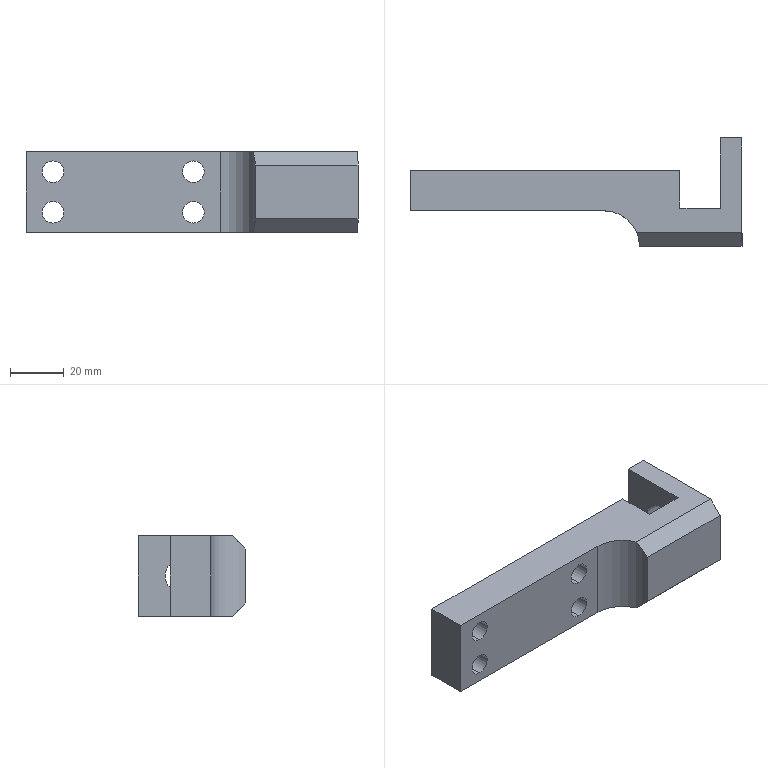Part | SolidWorks | features BaseBody 1 | 1 solid | 24 faces | box 123 x 40 x 30 mm | volume 62963 mm3 | plane 13 | cylinder 11 | commonest cylinder face diameters 8 x8 12 x2 26 x1
STEP:
#1=CARTESIAN_POINT('',(-340.,-80.,148.121));
#2=VERTEX_POINT('',#1);
#3=CARTESIAN_POINT('',(-340.,-80.,156.121));
#4=VERTEX_POINT('',#3);
#5=CARTESIAN_POINT('',(-340.,-80.,152.121));
#6=DIRECTION('',(0.,1.,0.));
#7=DIRECTION('',(0.,0.,-1.));
#8=AXIS2_PLACEMENT_3D('',#5,#6,#7);
#9=CIRCLE('',#8,4.);
#10=EDGE_CURVE('',#2,#4,#9,.T.);
#11=ORIENTED_EDGE('',*,*,#10,.T.);
#12=CARTESIAN_POINT('',(-340.,-95.,156.121));
#13=VERTEX_POINT('',#12);
#14=CARTESIAN_POINT('',(-340.,-95.,156.121));
#15=DIRECTION('',(0.,-1.,0.));
#16=VECTOR('',#15,1000.);
#17=LINE('',#14,#16);
#18=EDGE_CURVE('',#4,#13,#17,.T.);
#19=ORIENTED_EDGE('',*,*,#18,.T.);
#20=CARTESIAN_POINT('',(-340.,-95.,148.121));
#21=VERTEX_POINT('',#20);
#22=CARTESIAN_POINT('',(-340.,-95.,152.121));
#23=DIRECTION('',(0.,1.,0.));
#24=DIRECTION('',(0.,0.,-1.));
#25=AXIS2_PLACEMENT_3D('',#22,#23,#24);
#26=CIRCLE('',#25,4.);
#27=EDGE_CURVE('',#21,#13,#26,.T.);
#28=ORIENTED_EDGE('',*,*,#27,.F.);
#29=CARTESIAN_POINT('',(-340.,-95.,148.121));
#30=DIRECTION('',(0.,-1.,0.));
#31=VECTOR('',#30,1000.);
#32=LINE('',#29,#31);
#33=EDGE_CURVE('',#2,#21,#32,.T.);
#34=ORIENTED_EDGE('',*,*,#33,.F.);
#35=EDGE_LOOP('',(#11,#19,#28,#34));
#36=FACE_OUTER_BOUND('',#35,.T.);
#37=CARTESIAN_POINT('',(-340.,-95.,152.121));
#38=DIRECTION('',(0.,-1.,0.));
#39=DIRECTION('',(0.,0.,-1.));
#40=AXIS2_PLACEMENT_3D('',#37,#38,#39);
#41=CYLINDRICAL_SURFACE('',#40,4.);
#42=ADVANCED_FACE('',(#36),#41,.F.);
#43=CARTESIAN_POINT('',(-340.,-80.,133.121));
#44=VERTEX_POINT('',#43);
#45=CARTESIAN_POINT('',(-340.,-80.,141.121));
#46=VERTEX_POINT('',#45);
#47=CARTESIAN_POINT('',(-340.,-80.,137.121));
#48=DIRECTION('',(0.,1.,0.));
#49=DIRECTION('',(0.,0.,-1.));
#50=AXIS2_PLACEMENT_3D('',#47,#48,#49);
#51=CIRCLE('',#50,4.);
#52=EDGE_CURVE('',#44,#46,#51,.T.);
#53=ORIENTED_EDGE('',*,*,#52,.T.);
#54=CARTESIAN_POINT('',(-340.,-95.,141.121));
#55=VERTEX_POINT('',#54);
#56=CARTESIAN_POINT('',(-340.,-95.,141.121));
#57=DIRECTION('',(0.,-1.,0.));
#58=VECTOR('',#57,1000.);
#59=LINE('',#56,#58);
#60=EDGE_CURVE('',#46,#55,#59,.T.);
#61=ORIENTED_EDGE('',*,*,#60,.T.);
#62=CARTESIAN_POINT('',(-340.,-95.,133.121));
#63=VERTEX_POINT('',#62);
#64=CARTESIAN_POINT('',(-340.,-95.,137.121));
#65=DIRECTION('',(0.,1.,0.));
#66=DIRECTION('',(0.,0.,-1.));
#67=AXIS2_PLACEMENT_3D('',#64,#65,#66);
#68=CIRCLE('',#67,4.);
#69=EDGE_CURVE('',#63,#55,#68,.T.);
#70=ORIENTED_EDGE('',*,*,#69,.F.);
#71=CARTESIAN_POINT('',(-340.,-95.,133.121));
#72=DIRECTION('',(0.,-1.,0.));
#73=VECTOR('',#72,1000.);
#74=LINE('',#71,#73);
#75=EDGE_CURVE('',#44,#63,#74,.T.);
#76=ORIENTED_EDGE('',*,*,#75,.F.);
#77=EDGE_LOOP('',(#53,#61,#70,#76));
#78=FACE_OUTER_BOUND('',#77,.T.);
#79=CARTESIAN_POINT('',(-340.,-95.,137.121));
#80=DIRECTION('',(0.,-1.,0.));
#81=DIRECTION('',(0.,0.,-1.));
#82=AXIS2_PLACEMENT_3D('',#79,#80,#81);
#83=CYLINDRICAL_SURFACE('',#82,4.);
#84=ADVANCED_FACE('',(#78),#83,.F.);
#85=CARTESIAN_POINT('',(-288.,-80.,133.121));
#86=VERTEX_POINT('',#85);
#87=CARTESIAN_POINT('',(-288.,-80.,141.121));
#88=VERTEX_POINT('',#87);
#89=CARTESIAN_POINT('',(-288.,-80.,137.121));
#90=DIRECTION('',(0.,1.,0.));
#91=DIRECTION('',(0.,0.,-1.));
#92=AXIS2_PLACEMENT_3D('',#89,#90,#91);
#93=CIRCLE('',#92,4.);
#94=EDGE_CURVE('',#86,#88,#93,.T.);
#95=ORIENTED_EDGE('',*,*,#94,.T.);
#96=CARTESIAN_POINT('',(-288.,-95.,141.121));
#97=VERTEX_POINT('',#96);
#98=CARTESIAN_POINT('',(-288.,-95.,141.121));
#99=DIRECTION('',(0.,-1.,0.));
#100=VECTOR('',#99,1000.);
#101=LINE('',#98,#100);
#102=EDGE_CURVE('',#88,#97,#101,.T.);
#103=ORIENTED_EDGE('',*,*,#102,.T.);
#104=CARTESIAN_POINT('',(-288.,-95.,133.121));
#105=VERTEX_POINT('',#104);
#106=CARTESIAN_POINT('',(-288.,-95.,137.121));
#107=DIRECTION('',(0.,1.,0.));
#108=DIRECTION('',(0.,0.,-1.));
#109=AXIS2_PLACEMENT_3D('',#106,#107,#108);
#110=CIRCLE('',#109,4.);
#111=EDGE_CURVE('',#105,#97,#110,.T.);
#112=ORIENTED_EDGE('',*,*,#111,.F.);
#113=CARTESIAN_POINT('',(-288.,-95.,133.121));
#114=DIRECTION('',(0.,-1.,0.));
#115=VECTOR('',#114,1000.);
#116=LINE('',#113,#115);
#117=EDGE_CURVE('',#86,#105,#116,.T.);
#118=ORIENTED_EDGE('',*,*,#117,.F.);
#119=EDGE_LOOP('',(#95,#103,#112,#118));
#120=FACE_OUTER_BOUND('',#119,.T.);
#121=CARTESIAN_POINT('',(-288.,-95.,137.121));
#122=DIRECTION('',(0.,-1.,0.));
#123=DIRECTION('',(0.,0.,-1.));
#124=AXIS2_PLACEMENT_3D('',#121,#122,#123);
#125=CYLINDRICAL_SURFACE('',#124,4.);
#126=ADVANCED_FACE('',(#120),#125,.F.);
#127=CARTESIAN_POINT('',(-288.,-80.,148.121));
#128=VERTEX_POINT('',#127);
#129=CARTESIAN_POINT('',(-288.,-80.,156.121));
#130=VERTEX_POINT('',#129);
#131=CARTESIAN_POINT('',(-288.,-80.,152.121));
#132=DIRECTION('',(0.,1.,0.));
#133=DIRECTION('',(0.,0.,-1.));
#134=AXIS2_PLACEMENT_3D('',#131,#132,#133);
#135=CIRCLE('',#134,4.);
#136=EDGE_CURVE('',#128,#130,#135,.T.);
#137=ORIENTED_EDGE('',*,*,#136,.T.);
#138=CARTESIAN_POINT('',(-288.,-95.,156.121));
#139=VERTEX_POINT('',#138);
#140=CARTESIAN_POINT('',(-288.,-95.,156.121));
#141=DIRECTION('',(0.,-1.,0.));
#142=VECTOR('',#141,1000.);
#143=LINE('',#140,#142);
#144=EDGE_CURVE('',#130,#139,#143,.T.);
#145=ORIENTED_EDGE('',*,*,#144,.T.);
#146=CARTESIAN_POINT('',(-288.,-95.,148.121));
#147=VERTEX_POINT('',#146);
#148=CARTESIAN_POINT('',(-288.,-95.,152.121));
#149=DIRECTION('',(0.,1.,0.));
#150=DIRECTION('',(0.,0.,-1.));
#151=AXIS2_PLACEMENT_3D('',#148,#149,#150);
#152=CIRCLE('',#151,4.);
#153=EDGE_CURVE('',#147,#139,#152,.T.);
#154=ORIENTED_EDGE('',*,*,#153,.F.);
#155=CARTESIAN_POINT('',(-288.,-95.,148.121));
#156=DIRECTION('',(0.,-1.,0.));
#157=VECTOR('',#156,1000.);
#158=LINE('',#155,#157);
#159=EDGE_CURVE('',#128,#147,#158,.T.);
#160=ORIENTED_EDGE('',*,*,#159,.F.);
#161=EDGE_LOOP('',(#137,#145,#154,#160));
#162=FACE_OUTER_BOUND('',#161,.T.);
#163=CARTESIAN_POINT('',(-288.,-95.,152.121));
#164=DIRECTION('',(0.,-1.,0.));
#165=DIRECTION('',(0.,0.,-1.));
#166=AXIS2_PLACEMENT_3D('',#163,#164,#165);
#167=CYLINDRICAL_SURFACE('',#166,4.);
#168=ADVANCED_FACE('',(#162),#167,.F.);
#169=CARTESIAN_POINT('',(-235.,-84.,138.621));
#170=VERTEX_POINT('',#169);
#171=CARTESIAN_POINT('',(-235.,-84.,150.621));
#172=VERTEX_POINT('',#171);
#173=CARTESIAN_POINT('',(-235.,-84.,144.621));
#174=DIRECTION('',(-1.,0.,0.));
#175=DIRECTION('',(0.,0.,-1.));
#176=AXIS2_PLACEMENT_3D('',#173,#174,#175);
#177=CIRCLE('',#176,6.);
#178=EDGE_CURVE('',#170,#172,#177,.T.);
#179=ORIENTED_EDGE('',*,*,#178,.T.);
#180=CARTESIAN_POINT('',(-227.,-84.,150.621));
#181=VERTEX_POINT('',#180);
#182=CARTESIAN_POINT('',(-251.971,-84.,150.621));
#183=DIRECTION('',(1.,0.,0.));
#184=VECTOR('',#183,1000.);
#185=LINE('',#182,#184);
#186=EDGE_CURVE('',#172,#181,#185,.T.);
#187=ORIENTED_EDGE('',*,*,#186,.T.);
#188=CARTESIAN_POINT('',(-227.,-84.,138.621));
#189=VERTEX_POINT('',#188);
#190=CARTESIAN_POINT('',(-227.,-84.,144.621));
#191=DIRECTION('',(1.,0.,0.));
#192=DIRECTION('',(0.,0.,-1.));
#193=AXIS2_PLACEMENT_3D('',#190,#191,#192);
#194=CIRCLE('',#193,6.);
#195=EDGE_CURVE('',#181,#189,#194,.T.);
#196=ORIENTED_EDGE('',*,*,#195,.T.);
#197=CARTESIAN_POINT('',(-251.971,-84.,138.621));
#198=DIRECTION('',(1.,0.,0.));
#199=VECTOR('',#198,1000.);
#200=LINE('',#197,#199);
#201=EDGE_CURVE('',#170,#189,#200,.T.);
#202=ORIENTED_EDGE('',*,*,#201,.F.);
#203=EDGE_LOOP('',(#179,#187,#196,#202));
#204=FACE_OUTER_BOUND('',#203,.T.);
#205=CARTESIAN_POINT('',(-251.971,-84.,144.621));
#206=DIRECTION('',(1.,0.,0.));
#207=DIRECTION('',(0.,0.,-1.));
#208=AXIS2_PLACEMENT_3D('',#205,#206,#207);
#209=CYLINDRICAL_SURFACE('',#208,6.);
#210=ADVANCED_FACE('',(#204),#209,.F.);
#211=CARTESIAN_POINT('',(-350.,-80.,159.621));
#212=VERTEX_POINT('',#211);
#213=CARTESIAN_POINT('',(-350.,-80.,129.621));
#214=VERTEX_POINT('',#213);
#215=CARTESIAN_POINT('',(-350.,-80.,159.621));
#216=DIRECTION('',(0.,0.,-1.));
#217=VECTOR('',#216,1000.);
#218=LINE('',#215,#217);
#219=EDGE_CURVE('',#212,#214,#218,.T.);
#220=ORIENTED_EDGE('',*,*,#219,.F.);
#221=CARTESIAN_POINT('',(-250.,-80.,159.621));
#222=VERTEX_POINT('',#221);
#223=CARTESIAN_POINT('',(-350.,-80.,159.621));
#224=DIRECTION('',(-1.,0.,0.));
#225=VECTOR('',#224,1000.);
#226=LINE('',#223,#225);
#227=EDGE_CURVE('',#222,#212,#226,.T.);
#228=ORIENTED_EDGE('',*,*,#227,.F.);
#229=CARTESIAN_POINT('',(-250.,-80.,129.621));
#230=VERTEX_POINT('',#229);
#231=CARTESIAN_POINT('',(-250.,-80.,159.621));
#232=DIRECTION('',(0.,0.,1.));
#233=VECTOR('',#232,1000.);
#234=LINE('',#231,#233);
#235=EDGE_CURVE('',#230,#222,#234,.T.);
#236=ORIENTED_EDGE('',*,*,#235,.F.);
#237=CARTESIAN_POINT('',(-350.,-80.,129.621));
#238=DIRECTION('',(1.,0.,0.));
#239=VECTOR('',#238,1000.);
#240=LINE('',#237,#239);
#241=EDGE_CURVE('',#214,#230,#240,.T.);
#242=ORIENTED_EDGE('',*,*,#241,.F.);
#243=EDGE_LOOP('',(#220,#228,#236,#242));
#244=FACE_OUTER_BOUND('',#243,.T.);
#245=ORIENTED_EDGE('',*,*,#10,.F.);
#246=CARTESIAN_POINT('',(-340.,-80.,152.121));
#247=DIRECTION('',(0.,1.,0.));
#248=DIRECTION('',(0.,0.,-1.));
#249=AXIS2_PLACEMENT_3D('',#246,#247,#248);
#250=CIRCLE('',#249,4.);
#251=EDGE_CURVE('',#4,#2,#250,.T.);
#252=ORIENTED_EDGE('',*,*,#251,.F.);
#253=EDGE_LOOP('',(#245,#252));
#254=FACE_BOUND('',#253,.T.);
#255=ORIENTED_EDGE('',*,*,#52,.F.);
#256=CARTESIAN_POINT('',(-340.,-80.,137.121));
#257=DIRECTION('',(0.,1.,0.));
#258=DIRECTION('',(0.,0.,-1.));
#259=AXIS2_PLACEMENT_3D('',#256,#257,#258);
#260=CIRCLE('',#259,4.);
#261=EDGE_CURVE('',#46,#44,#260,.T.);
#262=ORIENTED_EDGE('',*,*,#261,.F.);
#263=EDGE_LOOP('',(#255,#262));
#264=FACE_BOUND('',#263,.T.);
#265=ORIENTED_EDGE('',*,*,#94,.F.);
#266=CARTESIAN_POINT('',(-288.,-80.,137.121));
#267=DIRECTION('',(0.,1.,0.));
#268=DIRECTION('',(0.,0.,-1.));
#269=AXIS2_PLACEMENT_3D('',#266,#267,#268);
#270=CIRCLE('',#269,4.);
#271=EDGE_CURVE('',#88,#86,#270,.T.);
#272=ORIENTED_EDGE('',*,*,#271,.F.);
#273=EDGE_LOOP('',(#265,#272));
#274=FACE_BOUND('',#273,.T.);
#275=ORIENTED_EDGE('',*,*,#136,.F.);
#276=CARTESIAN_POINT('',(-288.,-80.,152.121));
#277=DIRECTION('',(0.,1.,0.));
#278=DIRECTION('',(0.,0.,-1.));
#279=AXIS2_PLACEMENT_3D('',#276,#277,#278);
#280=CIRCLE('',#279,4.);
#281=EDGE_CURVE('',#130,#128,#280,.T.);
#282=ORIENTED_EDGE('',*,*,#281,.F.);
#283=EDGE_LOOP('',(#275,#282));
#284=FACE_BOUND('',#283,.T.);
#285=CARTESIAN_POINT('',(-350.,-80.,159.621));
#286=DIRECTION('',(0.,-1.,0.));
#287=DIRECTION('',(0.,0.,-1.));
#288=AXIS2_PLACEMENT_3D('',#285,#286,#287);
#289=PLANE('',#288);
#290=ADVANCED_FACE('',(#244,#254,#264,#274,#284),#289,.F.);
#291=CARTESIAN_POINT('',(-266.,-103.,129.621));
#292=VERTEX_POINT('',#291);
#293=CARTESIAN_POINT('',(-227.,-103.,129.621));
#294=VERTEX_POINT('',#293);
#295=CARTESIAN_POINT('',(-251.867,-103.,129.621));
#296=DIRECTION('',(1.,0.,0.));
#297=VECTOR('',#296,1000.);
#298=LINE('',#295,#297);
#299=EDGE_CURVE('',#292,#294,#298,.T.);
#300=ORIENTED_EDGE('',*,*,#299,.F.);
#301=CARTESIAN_POINT('',(-278.,-95.,129.621));
#302=VERTEX_POINT('',#301);
#303=CARTESIAN_POINT('',(-278.,-108.,129.621));
#304=DIRECTION('',(0.,0.,-1.));
#305=DIRECTION('',(1.,0.,0.));
#306=AXIS2_PLACEMENT_3D('',#303,#304,#305);
#307=CIRCLE('',#306,13.);
#308=EDGE_CURVE('',#302,#292,#307,.T.);
#309=ORIENTED_EDGE('',*,*,#308,.F.);
#310=CARTESIAN_POINT('',(-350.,-95.,129.621));
#311=VERTEX_POINT('',#310);
#312=CARTESIAN_POINT('',(-251.867,-95.,129.621));
#313=DIRECTION('',(1.,0.,0.));
#314=VECTOR('',#313,1000.);
#315=LINE('',#312,#314);
#316=EDGE_CURVE('',#311,#302,#315,.T.);
#317=ORIENTED_EDGE('',*,*,#316,.F.);
#318=CARTESIAN_POINT('',(-350.,-82.6,129.621));
#319=DIRECTION('',(0.,-1.,0.));
#320=VECTOR('',#319,1000.);
#321=LINE('',#318,#320);
#322=EDGE_CURVE('',#214,#311,#321,.T.);
#323=ORIENTED_EDGE('',*,*,#322,.F.);
#324=ORIENTED_EDGE('',*,*,#241,.T.);
#325=CARTESIAN_POINT('',(-250.,-94.,129.621));
#326=VERTEX_POINT('',#325);
#327=CARTESIAN_POINT('',(-250.,-82.6,129.621));
#328=DIRECTION('',(0.,1.,0.));
#329=VECTOR('',#328,1000.);
#330=LINE('',#327,#329);
#331=EDGE_CURVE('',#326,#230,#330,.T.);
#332=ORIENTED_EDGE('',*,*,#331,.F.);
#333=CARTESIAN_POINT('',(-235.,-94.,129.621));
#334=VERTEX_POINT('',#333);
#335=CARTESIAN_POINT('',(-251.867,-94.,129.621));
#336=DIRECTION('',(-1.,0.,0.));
#337=VECTOR('',#336,1000.);
#338=LINE('',#335,#337);
#339=EDGE_CURVE('',#334,#326,#338,.T.);
#340=ORIENTED_EDGE('',*,*,#339,.F.);
#341=CARTESIAN_POINT('',(-235.,-68.,129.621));
#342=VERTEX_POINT('',#341);
#343=CARTESIAN_POINT('',(-235.,-82.6,129.621));
#344=DIRECTION('',(0.,-1.,0.));
#345=VECTOR('',#344,1000.);
#346=LINE('',#343,#345);
#347=EDGE_CURVE('',#342,#334,#346,.T.);
#348=ORIENTED_EDGE('',*,*,#347,.F.);
#349=CARTESIAN_POINT('',(-227.,-68.,129.621));
#350=VERTEX_POINT('',#349);
#351=CARTESIAN_POINT('',(-251.867,-68.,129.621));
#352=DIRECTION('',(-1.,0.,0.));
#353=VECTOR('',#352,1000.);
#354=LINE('',#351,#353);
#355=EDGE_CURVE('',#350,#342,#354,.T.);
#356=ORIENTED_EDGE('',*,*,#355,.F.);
#357=CARTESIAN_POINT('',(-227.,-82.6,129.621));
#358=DIRECTION('',(0.,1.,0.));
#359=VECTOR('',#358,1000.);
#360=LINE('',#357,#359);
#361=EDGE_CURVE('',#294,#350,#360,.T.);
#362=ORIENTED_EDGE('',*,*,#361,.F.);
#363=EDGE_LOOP('',(#300,#309,#317,#323,#324,#332,#340,#348,#356,#362));
#364=FACE_OUTER_BOUND('',#363,.T.);
#365=CARTESIAN_POINT('',(-251.867,-82.6,129.621));
#366=DIRECTION('',(0.,0.,1.));
#367=DIRECTION('',(1.,0.,0.));
#368=AXIS2_PLACEMENT_3D('',#365,#366,#367);
#369=PLANE('',#368);
#370=ADVANCED_FACE('',(#364),#369,.F.);
#371=CARTESIAN_POINT('',(-350.,-95.,159.621));
#372=VERTEX_POINT('',#371);
#373=CARTESIAN_POINT('',(-350.,-95.,159.621));
#374=DIRECTION('',(0.,0.,-1.));
#375=VECTOR('',#374,1000.);
#376=LINE('',#373,#375);
#377=EDGE_CURVE('',#372,#311,#376,.T.);
#378=ORIENTED_EDGE('',*,*,#377,.F.);
#379=CARTESIAN_POINT('',(-350.,-80.,159.621));
#380=DIRECTION('',(0.,-1.,0.));
#381=VECTOR('',#380,1000.);
#382=LINE('',#379,#381);
#383=EDGE_CURVE('',#212,#372,#382,.T.);
#384=ORIENTED_EDGE('',*,*,#383,.F.);
#385=ORIENTED_EDGE('',*,*,#219,.T.);
#386=ORIENTED_EDGE('',*,*,#322,.T.);
#387=EDGE_LOOP('',(#378,#384,#385,#386));
#388=FACE_OUTER_BOUND('',#387,.T.);
#389=CARTESIAN_POINT('',(-350.,-80.,159.621));
#390=DIRECTION('',(1.,0.,0.));
#391=DIRECTION('',(0.,0.,-1.));
#392=AXIS2_PLACEMENT_3D('',#389,#390,#391);
#393=PLANE('',#392);
#394=ADVANCED_FACE('',(#388),#393,.F.);
#395=ORIENTED_EDGE('',*,*,#383,.T.);
#396=CARTESIAN_POINT('',(-278.,-95.,159.621));
#397=VERTEX_POINT('',#396);
#398=CARTESIAN_POINT('',(-251.867,-95.,159.621));
#399=DIRECTION('',(1.,0.,0.));
#400=VECTOR('',#399,1000.);
#401=LINE('',#398,#400);
#402=EDGE_CURVE('',#372,#397,#401,.T.);
#403=ORIENTED_EDGE('',*,*,#402,.T.);
#404=CARTESIAN_POINT('',(-266.,-103.,159.621));
#405=VERTEX_POINT('',#404);
#406=CARTESIAN_POINT('',(-278.,-108.,159.621));
#407=DIRECTION('',(0.,0.,-1.));
#408=DIRECTION('',(1.,0.,0.));
#409=AXIS2_PLACEMENT_3D('',#406,#407,#408);
#410=CIRCLE('',#409,13.);
#411=EDGE_CURVE('',#397,#405,#410,.T.);
#412=ORIENTED_EDGE('',*,*,#411,.T.);
#413=CARTESIAN_POINT('',(-227.,-103.,159.621));
#414=VERTEX_POINT('',#413);
#415=CARTESIAN_POINT('',(-251.867,-103.,159.621));
#416=DIRECTION('',(1.,0.,0.));
#417=VECTOR('',#416,1000.);
#418=LINE('',#415,#417);
#419=EDGE_CURVE('',#405,#414,#418,.T.);
#420=ORIENTED_EDGE('',*,*,#419,.T.);
#421=CARTESIAN_POINT('',(-227.,-68.,159.621));
#422=VERTEX_POINT('',#421);
#423=CARTESIAN_POINT('',(-227.,-82.6,159.621));
#424=DIRECTION('',(0.,1.,0.));
#425=VECTOR('',#424,1000.);
#426=LINE('',#423,#425);
#427=EDGE_CURVE('',#414,#422,#426,.T.);
#428=ORIENTED_EDGE('',*,*,#427,.T.);
#429=CARTESIAN_POINT('',(-235.,-68.,159.621));
#430=VERTEX_POINT('',#429);
#431=CARTESIAN_POINT('',(-251.867,-68.,159.621));
#432=DIRECTION('',(-1.,0.,0.));
#433=VECTOR('',#432,1000.);
#434=LINE('',#431,#433);
#435=EDGE_CURVE('',#422,#430,#434,.T.);
#436=ORIENTED_EDGE('',*,*,#435,.T.);
#437=CARTESIAN_POINT('',(-235.,-94.,159.621));
#438=VERTEX_POINT('',#437);
#439=CARTESIAN_POINT('',(-235.,-82.6,159.621));
#440=DIRECTION('',(0.,-1.,0.));
#441=VECTOR('',#440,1000.);
#442=LINE('',#439,#441);
#443=EDGE_CURVE('',#430,#438,#442,.T.);
#444=ORIENTED_EDGE('',*,*,#443,.T.);
#445=CARTESIAN_POINT('',(-250.,-94.,159.621));
#446=VERTEX_POINT('',#445);
#447=CARTESIAN_POINT('',(-251.867,-94.,159.621));
#448=DIRECTION('',(-1.,0.,0.));
#449=VECTOR('',#448,1000.);
#450=LINE('',#447,#449);
#451=EDGE_CURVE('',#438,#446,#450,.T.);
#452=ORIENTED_EDGE('',*,*,#451,.T.);
#453=CARTESIAN_POINT('',(-250.,-82.6,159.621));
#454=DIRECTION('',(0.,1.,0.));
#455=VECTOR('',#454,1000.);
#456=LINE('',#453,#455);
#457=EDGE_CURVE('',#446,#222,#456,.T.);
#458=ORIENTED_EDGE('',*,*,#457,.T.);
#459=ORIENTED_EDGE('',*,*,#227,.T.);
#460=EDGE_LOOP('',(#395,#403,#412,#420,#428,#436,#444,#452,#458,#459));
#461=FACE_OUTER_BOUND('',#460,.T.);
#462=CARTESIAN_POINT('',(-251.867,-82.6,159.621));
#463=DIRECTION('',(0.,0.,1.));
#464=DIRECTION('',(1.,0.,0.));
#465=AXIS2_PLACEMENT_3D('',#462,#463,#464);
#466=PLANE('',#465);
#467=ADVANCED_FACE('',(#461),#466,.T.);
#468=ORIENTED_EDGE('',*,*,#235,.T.);
#469=ORIENTED_EDGE('',*,*,#457,.F.);
#470=CARTESIAN_POINT('',(-250.,-94.,159.621));
#471=DIRECTION('',(0.,0.,1.));
#472=VECTOR('',#471,1000.);
#473=LINE('',#470,#472);
#474=EDGE_CURVE('',#326,#446,#473,.T.);
#475=ORIENTED_EDGE('',*,*,#474,.F.);
#476=ORIENTED_EDGE('',*,*,#331,.T.);
#477=EDGE_LOOP('',(#468,#469,#475,#476));
#478=FACE_OUTER_BOUND('',#477,.T.);
#479=CARTESIAN_POINT('',(-250.,-80.,159.621));
#480=DIRECTION('',(-1.,0.,0.));
#481=DIRECTION('',(0.,0.,1.));
#482=AXIS2_PLACEMENT_3D('',#479,#480,#481);
#483=PLANE('',#482);
#484=ADVANCED_FACE('',(#478),#483,.F.);
#485=ORIENTED_EDGE('',*,*,#18,.F.);
#486=ORIENTED_EDGE('',*,*,#251,.T.);
#487=ORIENTED_EDGE('',*,*,#33,.T.);
#488=CARTESIAN_POINT('',(-340.,-95.,152.121));
#489=DIRECTION('',(0.,1.,0.));
#490=DIRECTION('',(0.,0.,-1.));
#491=AXIS2_PLACEMENT_3D('',#488,#489,#490);
#492=CIRCLE('',#491,4.);
#493=EDGE_CURVE('',#13,#21,#492,.T.);
#494=ORIENTED_EDGE('',*,*,#493,.F.);
#495=EDGE_LOOP('',(#485,#486,#487,#494));
#496=FACE_OUTER_BOUND('',#495,.T.);
#497=CARTESIAN_POINT('',(-340.,-95.,152.121));
#498=DIRECTION('',(0.,-1.,0.));
#499=DIRECTION('',(0.,0.,-1.));
#500=AXIS2_PLACEMENT_3D('',#497,#498,#499);
#501=CYLINDRICAL_SURFACE('',#500,4.);
#502=ADVANCED_FACE('',(#496),#501,.F.);
#503=ORIENTED_EDGE('',*,*,#60,.F.);
#504=ORIENTED_EDGE('',*,*,#261,.T.);
#505=ORIENTED_EDGE('',*,*,#75,.T.);
#506=CARTESIAN_POINT('',(-340.,-95.,137.121));
#507=DIRECTION('',(0.,1.,0.));
#508=DIRECTION('',(0.,0.,-1.));
#509=AXIS2_PLACEMENT_3D('',#506,#507,#508);
#510=CIRCLE('',#509,4.);
#511=EDGE_CURVE('',#55,#63,#510,.T.);
#512=ORIENTED_EDGE('',*,*,#511,.F.);
#513=EDGE_LOOP('',(#503,#504,#505,#512));
#514=FACE_OUTER_BOUND('',#513,.T.);
#515=CARTESIAN_POINT('',(-340.,-95.,137.121));
#516=DIRECTION('',(0.,-1.,0.));
#517=DIRECTION('',(0.,0.,-1.));
#518=AXIS2_PLACEMENT_3D('',#515,#516,#517);
#519=CYLINDRICAL_SURFACE('',#518,4.);
#520=ADVANCED_FACE('',(#514),#519,.F.);
#521=ORIENTED_EDGE('',*,*,#102,.F.);
#522=ORIENTED_EDGE('',*,*,#271,.T.);
#523=ORIENTED_EDGE('',*,*,#117,.T.);
#524=CARTESIAN_POINT('',(-288.,-95.,137.121));
#525=DIRECTION('',(0.,1.,0.));
#526=DIRECTION('',(0.,0.,-1.));
#527=AXIS2_PLACEMENT_3D('',#524,#525,#526);
#528=CIRCLE('',#527,4.);
#529=EDGE_CURVE('',#97,#105,#528,.T.);
#530=ORIENTED_EDGE('',*,*,#529,.F.);
#531=EDGE_LOOP('',(#521,#522,#523,#530));
#532=FACE_OUTER_BOUND('',#531,.T.);
#533=CARTESIAN_POINT('',(-288.,-95.,137.121));
#534=DIRECTION('',(0.,-1.,0.));
#535=DIRECTION('',(0.,0.,-1.));
#536=AXIS2_PLACEMENT_3D('',#533,#534,#535);
#537=CYLINDRICAL_SURFACE('',#536,4.);
#538=ADVANCED_FACE('',(#532),#537,.F.);
#539=ORIENTED_EDGE('',*,*,#144,.F.);
#540=ORIENTED_EDGE('',*,*,#281,.T.);
#541=ORIENTED_EDGE('',*,*,#159,.T.);
#542=CARTESIAN_POINT('',(-288.,-95.,152.121));
#543=DIRECTION('',(0.,1.,0.));
#544=DIRECTION('',(0.,0.,-1.));
#545=AXIS2_PLACEMENT_3D('',#542,#543,#544);
#546=CIRCLE('',#545,4.);
#547=EDGE_CURVE('',#139,#147,#546,.T.);
#548=ORIENTED_EDGE('',*,*,#547,.F.);
#549=EDGE_LOOP('',(#539,#540,#541,#548));
#550=FACE_OUTER_BOUND('',#549,.T.);
#551=CARTESIAN_POINT('',(-288.,-95.,152.121));
#552=DIRECTION('',(0.,-1.,0.));
#553=DIRECTION('',(0.,0.,-1.));
#554=AXIS2_PLACEMENT_3D('',#551,#552,#553);
#555=CYLINDRICAL_SURFACE('',#554,4.);
#556=ADVANCED_FACE('',(#550),#555,.F.);
#557=CARTESIAN_POINT('',(-227.,-108.,154.621));
#558=VERTEX_POINT('',#557);
#559=CARTESIAN_POINT('',(-227.,-108.,154.621));
#560=DIRECTION('',(0.,0.7071,0.7071));
#561=VECTOR('',#560,1000.);
#562=LINE('',#559,#561);
#563=EDGE_CURVE('',#558,#414,#562,.T.);
#564=ORIENTED_EDGE('',*,*,#563,.F.);
#565=CARTESIAN_POINT('',(-227.,-108.,134.621));
#566=VERTEX_POINT('',#565);
#567=CARTESIAN_POINT('',(-227.,-108.,159.621));
#568=DIRECTION('',(0.,0.,1.));
#569=VECTOR('',#568,1000.);
#570=LINE('',#567,#569);
#571=EDGE_CURVE('',#566,#558,#570,.T.);
#572=ORIENTED_EDGE('',*,*,#571,.F.);
#573=CARTESIAN_POINT('',(-227.,-103.,129.621));
#574=DIRECTION('',(0.,-0.7071,0.7071));
#575=VECTOR('',#574,1000.);
#576=LINE('',#573,#575);
#577=EDGE_CURVE('',#294,#566,#576,.T.);
#578=ORIENTED_EDGE('',*,*,#577,.F.);
#579=ORIENTED_EDGE('',*,*,#361,.T.);
#580=CARTESIAN_POINT('',(-227.,-68.,159.621));
#581=DIRECTION('',(0.,0.,-1.));
#582=VECTOR('',#581,1000.);
#583=LINE('',#580,#582);
#584=EDGE_CURVE('',#422,#350,#583,.T.);
#585=ORIENTED_EDGE('',*,*,#584,.F.);
#586=ORIENTED_EDGE('',*,*,#427,.F.);
#587=EDGE_LOOP('',(#564,#572,#578,#579,#585,#586));
#588=FACE_OUTER_BOUND('',#587,.T.);
#589=CARTESIAN_POINT('',(-227.,-84.,144.621));
#590=DIRECTION('',(1.,0.,0.));
#591=DIRECTION('',(0.,0.,-1.));
#592=AXIS2_PLACEMENT_3D('',#589,#590,#591);
#593=CIRCLE('',#592,6.);
#594=EDGE_CURVE('',#189,#181,#593,.T.);
#595=ORIENTED_EDGE('',*,*,#594,.F.);
#596=ORIENTED_EDGE('',*,*,#195,.F.);
#597=EDGE_LOOP('',(#595,#596));
#598=FACE_BOUND('',#597,.T.);
#599=CARTESIAN_POINT('',(-227.,-93.,159.621));
#600=DIRECTION('',(-1.,0.,0.));
#601=DIRECTION('',(0.,0.,1.));
#602=AXIS2_PLACEMENT_3D('',#599,#600,#601);
#603=PLANE('',#602);
#604=ADVANCED_FACE('',(#588,#598),#603,.F.);
#605=ORIENTED_EDGE('',*,*,#299,.T.);
#606=ORIENTED_EDGE('',*,*,#577,.T.);
#607=CARTESIAN_POINT('',(-265.,-108.,134.621));
#608=VERTEX_POINT('',#607);
#609=CARTESIAN_POINT('',(-265.,-108.,134.621));
#610=DIRECTION('',(1.,0.,0.));
#611=VECTOR('',#610,1000.);
#612=LINE('',#609,#611);
#613=EDGE_CURVE('',#608,#566,#612,.T.);
#614=ORIENTED_EDGE('',*,*,#613,.F.);
#615=CARTESIAN_POINT('',(-266.,-103.,129.621));
#616=CARTESIAN_POINT('',(-265.338,-104.59,131.211));
#617=CARTESIAN_POINT('',(-265.,-106.278,132.899));
#618=CARTESIAN_POINT('',(-265.,-108.,134.621));
#619=(BOUNDED_CURVE()B_SPLINE_CURVE(3,(#615,#616,#617,#618),.UNSPECIFIED.,.F.,.F.)B_SPLINE_CURVE_WITH_KNOTS((4,4),(4.318,4.712),.UNSPECIFIED.)CURVE()GEOMETRIC_REPRESENTATION_ITEM()RATIONAL_B_SPLINE_CURVE((1.,0.9871,0.9871,1.))REPRESENTATION_ITEM(''));
#620=EDGE_CURVE('',#292,#608,#619,.T.);
#621=ORIENTED_EDGE('',*,*,#620,.F.);
#622=EDGE_LOOP('',(#605,#606,#614,#621));
#623=FACE_OUTER_BOUND('',#622,.T.);
#624=CARTESIAN_POINT('',(-265.,-108.,134.621));
#625=DIRECTION('',(0.,0.7071,0.7071));
#626=DIRECTION('',(0.,-0.7071,0.7071));
#627=AXIS2_PLACEMENT_3D('',#624,#625,#626);
#628=PLANE('',#627);
#629=ADVANCED_FACE('',(#623),#628,.F.);
#630=CARTESIAN_POINT('',(-265.,-108.,154.621));
#631=VERTEX_POINT('',#630);
#632=CARTESIAN_POINT('',(-266.,-103.,159.621));
#633=CARTESIAN_POINT('',(-265.338,-104.59,158.032));
#634=CARTESIAN_POINT('',(-265.,-106.278,156.343));
#635=CARTESIAN_POINT('',(-265.,-108.,154.621));
#636=(BOUNDED_CURVE()B_SPLINE_CURVE(3,(#632,#633,#634,#635),.UNSPECIFIED.,.F.,.F.)B_SPLINE_CURVE_WITH_KNOTS((4,4),(1.176,1.571),.UNSPECIFIED.)CURVE()GEOMETRIC_REPRESENTATION_ITEM()RATIONAL_B_SPLINE_CURVE((1.,0.9871,0.9871,1.))REPRESENTATION_ITEM(''));
#637=EDGE_CURVE('',#405,#631,#636,.T.);
#638=ORIENTED_EDGE('',*,*,#637,.F.);
#639=ORIENTED_EDGE('',*,*,#411,.F.);
#640=CARTESIAN_POINT('',(-278.,-95.,159.621));
#641=DIRECTION('',(0.,0.,1.));
#642=VECTOR('',#641,1000.);
#643=LINE('',#640,#642);
#644=EDGE_CURVE('',#302,#397,#643,.T.);
#645=ORIENTED_EDGE('',*,*,#644,.F.);
#646=ORIENTED_EDGE('',*,*,#308,.T.);
#647=ORIENTED_EDGE('',*,*,#620,.T.);
#648=CARTESIAN_POINT('',(-265.,-108.,159.621));
#649=DIRECTION('',(0.,0.,-1.));
#650=VECTOR('',#649,1000.);
#651=LINE('',#648,#650);
#652=EDGE_CURVE('',#631,#608,#651,.T.);
#653=ORIENTED_EDGE('',*,*,#652,.F.);
#654=EDGE_LOOP('',(#638,#639,#645,#646,#647,#653));
#655=FACE_OUTER_BOUND('',#654,.T.);
#656=CARTESIAN_POINT('',(-278.,-108.,159.621));
#657=DIRECTION('',(0.,0.,1.));
#658=DIRECTION('',(1.,0.,0.));
#659=AXIS2_PLACEMENT_3D('',#656,#657,#658);
#660=CYLINDRICAL_SURFACE('',#659,13.);
#661=ADVANCED_FACE('',(#655),#660,.F.);
#662=ORIENTED_EDGE('',*,*,#644,.T.);
#663=ORIENTED_EDGE('',*,*,#402,.F.);
#664=ORIENTED_EDGE('',*,*,#377,.T.);
#665=ORIENTED_EDGE('',*,*,#316,.T.);
#666=EDGE_LOOP('',(#662,#663,#664,#665));
#667=FACE_OUTER_BOUND('',#666,.T.);
#668=ORIENTED_EDGE('',*,*,#27,.T.);
#669=ORIENTED_EDGE('',*,*,#493,.T.);
#670=EDGE_LOOP('',(#668,#669));
#671=FACE_BOUND('',#670,.T.);
#672=ORIENTED_EDGE('',*,*,#69,.T.);
#673=ORIENTED_EDGE('',*,*,#511,.T.);
#674=EDGE_LOOP('',(#672,#673));
#675=FACE_BOUND('',#674,.T.);
#676=ORIENTED_EDGE('',*,*,#111,.T.);
#677=ORIENTED_EDGE('',*,*,#529,.T.);
#678=EDGE_LOOP('',(#676,#677));
#679=FACE_BOUND('',#678,.T.);
#680=ORIENTED_EDGE('',*,*,#153,.T.);
#681=ORIENTED_EDGE('',*,*,#547,.T.);
#682=EDGE_LOOP('',(#680,#681));
#683=FACE_BOUND('',#682,.T.);
#684=CARTESIAN_POINT('',(-350.,-95.,159.621));
#685=DIRECTION('',(0.,1.,0.));
#686=DIRECTION('',(0.,0.,1.));
#687=AXIS2_PLACEMENT_3D('',#684,#685,#686);
#688=PLANE('',#687);
#689=ADVANCED_FACE('',(#667,#671,#675,#679,#683),#688,.F.);
#690=ORIENTED_EDGE('',*,*,#474,.T.);
#691=ORIENTED_EDGE('',*,*,#451,.F.);
#692=CARTESIAN_POINT('',(-235.,-94.,159.621));
#693=DIRECTION('',(0.,0.,1.));
#694=VECTOR('',#693,1000.);
#695=LINE('',#692,#694);
#696=EDGE_CURVE('',#334,#438,#695,.T.);
#697=ORIENTED_EDGE('',*,*,#696,.F.);
#698=ORIENTED_EDGE('',*,*,#339,.T.);
#699=EDGE_LOOP('',(#690,#691,#697,#698));
#700=FACE_OUTER_BOUND('',#699,.T.);
#701=CARTESIAN_POINT('',(-250.,-94.,159.621));
#702=DIRECTION('',(0.,-1.,0.));
#703=DIRECTION('',(0.,0.,-1.));
#704=AXIS2_PLACEMENT_3D('',#701,#702,#703);
#705=PLANE('',#704);
#706=ADVANCED_FACE('',(#700),#705,.F.);
#707=ORIENTED_EDGE('',*,*,#696,.T.);
#708=ORIENTED_EDGE('',*,*,#443,.F.);
#709=CARTESIAN_POINT('',(-235.,-68.,159.621));
#710=DIRECTION('',(0.,0.,1.));
#711=VECTOR('',#710,1000.);
#712=LINE('',#709,#711);
#713=EDGE_CURVE('',#342,#430,#712,.T.);
#714=ORIENTED_EDGE('',*,*,#713,.F.);
#715=ORIENTED_EDGE('',*,*,#347,.T.);
#716=EDGE_LOOP('',(#707,#708,#714,#715));
#717=FACE_OUTER_BOUND('',#716,.T.);
#718=ORIENTED_EDGE('',*,*,#178,.F.);
#719=CARTESIAN_POINT('',(-235.,-84.,144.621));
#720=DIRECTION('',(-1.,0.,0.));
#721=DIRECTION('',(0.,0.,-1.));
#722=AXIS2_PLACEMENT_3D('',#719,#720,#721);
#723=CIRCLE('',#722,6.);
#724=EDGE_CURVE('',#172,#170,#723,.T.);
#725=ORIENTED_EDGE('',*,*,#724,.F.);
#726=EDGE_LOOP('',(#718,#725));
#727=FACE_BOUND('',#726,.T.);
#728=CARTESIAN_POINT('',(-235.,-94.,159.621));
#729=DIRECTION('',(1.,0.,0.));
#730=DIRECTION('',(0.,0.,-1.));
#731=AXIS2_PLACEMENT_3D('',#728,#729,#730);
#732=PLANE('',#731);
#733=ADVANCED_FACE('',(#717,#727),#732,.F.);
#734=ORIENTED_EDGE('',*,*,#713,.T.);
#735=ORIENTED_EDGE('',*,*,#435,.F.);
#736=ORIENTED_EDGE('',*,*,#584,.T.);
#737=ORIENTED_EDGE('',*,*,#355,.T.);
#738=EDGE_LOOP('',(#734,#735,#736,#737));
#739=FACE_OUTER_BOUND('',#738,.T.);
#740=CARTESIAN_POINT('',(-227.,-68.,159.621));
#741=DIRECTION('',(0.,-1.,0.));
#742=DIRECTION('',(0.,0.,-1.));
#743=AXIS2_PLACEMENT_3D('',#740,#741,#742);
#744=PLANE('',#743);
#745=ADVANCED_FACE('',(#739),#744,.F.);
#746=ORIENTED_EDGE('',*,*,#563,.T.);
#747=ORIENTED_EDGE('',*,*,#419,.F.);
#748=ORIENTED_EDGE('',*,*,#637,.T.);
#749=CARTESIAN_POINT('',(-251.867,-108.,154.621));
#750=DIRECTION('',(1.,0.,0.));
#751=VECTOR('',#750,1000.);
#752=LINE('',#749,#751);
#753=EDGE_CURVE('',#631,#558,#752,.T.);
#754=ORIENTED_EDGE('',*,*,#753,.T.);
#755=EDGE_LOOP('',(#746,#747,#748,#754));
#756=FACE_OUTER_BOUND('',#755,.T.);
#757=CARTESIAN_POINT('',(-251.867,-103.,159.621));
#758=DIRECTION('',(0.,-0.7071,0.7071));
#759=DIRECTION('',(0.,-0.7071,-0.7071));
#760=AXIS2_PLACEMENT_3D('',#757,#758,#759);
#761=PLANE('',#760);
#762=ADVANCED_FACE('',(#756),#761,.T.);
#763=ORIENTED_EDGE('',*,*,#753,.F.);
#764=ORIENTED_EDGE('',*,*,#652,.T.);
#765=ORIENTED_EDGE('',*,*,#613,.T.);
#766=ORIENTED_EDGE('',*,*,#571,.T.);
#767=EDGE_LOOP('',(#763,#764,#765,#766));
#768=FACE_OUTER_BOUND('',#767,.T.);
#769=CARTESIAN_POINT('',(-265.,-108.,159.621));
#770=DIRECTION('',(0.,1.,0.));
#771=DIRECTION('',(0.,0.,1.));
#772=AXIS2_PLACEMENT_3D('',#769,#770,#771);
#773=PLANE('',#772);
#774=ADVANCED_FACE('',(#768),#773,.F.);
#775=ORIENTED_EDGE('',*,*,#186,.F.);
#776=ORIENTED_EDGE('',*,*,#724,.T.);
#777=ORIENTED_EDGE('',*,*,#201,.T.);
#778=ORIENTED_EDGE('',*,*,#594,.T.);
#779=EDGE_LOOP('',(#775,#776,#777,#778));
#780=FACE_OUTER_BOUND('',#779,.T.);
#781=CARTESIAN_POINT('',(-251.971,-84.,144.621));
#782=DIRECTION('',(1.,0.,0.));
#783=DIRECTION('',(0.,0.,-1.));
#784=AXIS2_PLACEMENT_3D('',#781,#782,#783);
#785=CYLINDRICAL_SURFACE('',#784,6.);
#786=ADVANCED_FACE('',(#780),#785,.F.);
#787=CLOSED_SHELL('',(#42,#84,#126,#168,#210,#290,#370,#394,#467,#484,#502,#520,#538,#556,#604,#629,#661,#689,#706,#733,#745,#762,#774,#786));
#788=MANIFOLD_SOLID_BREP('',#787);
#789=CARTESIAN_POINT('',(0.,0.,0.));
#790=DIRECTION('',(0.,0.,1.));
#791=DIRECTION('',(1.,0.,0.));
#792=AXIS2_PLACEMENT_3D('',#789,#790,#791);
#793=(LENGTH_UNIT()NAMED_UNIT(*)SI_UNIT(.MILLI.,.METRE.));
#794=UNCERTAINTY_MEASURE_WITH_UNIT(LENGTH_MEASURE(0.00001),#793,'','');
#795=(NAMED_UNIT(*)PLANE_ANGLE_UNIT()SI_UNIT($,.RADIAN.));
#796=(NAMED_UNIT(*)SI_UNIT($,.STERADIAN.)SOLID_ANGLE_UNIT());
#797=(GEOMETRIC_REPRESENTATION_CONTEXT(3)GLOBAL_UNCERTAINTY_ASSIGNED_CONTEXT((#794))GLOBAL_UNIT_ASSIGNED_CONTEXT((#793,#795,#796))REPRESENTATION_CONTEXT('',''));
#798=ADVANCED_BREP_SHAPE_REPRESENTATION('',(#788,#792),#797);